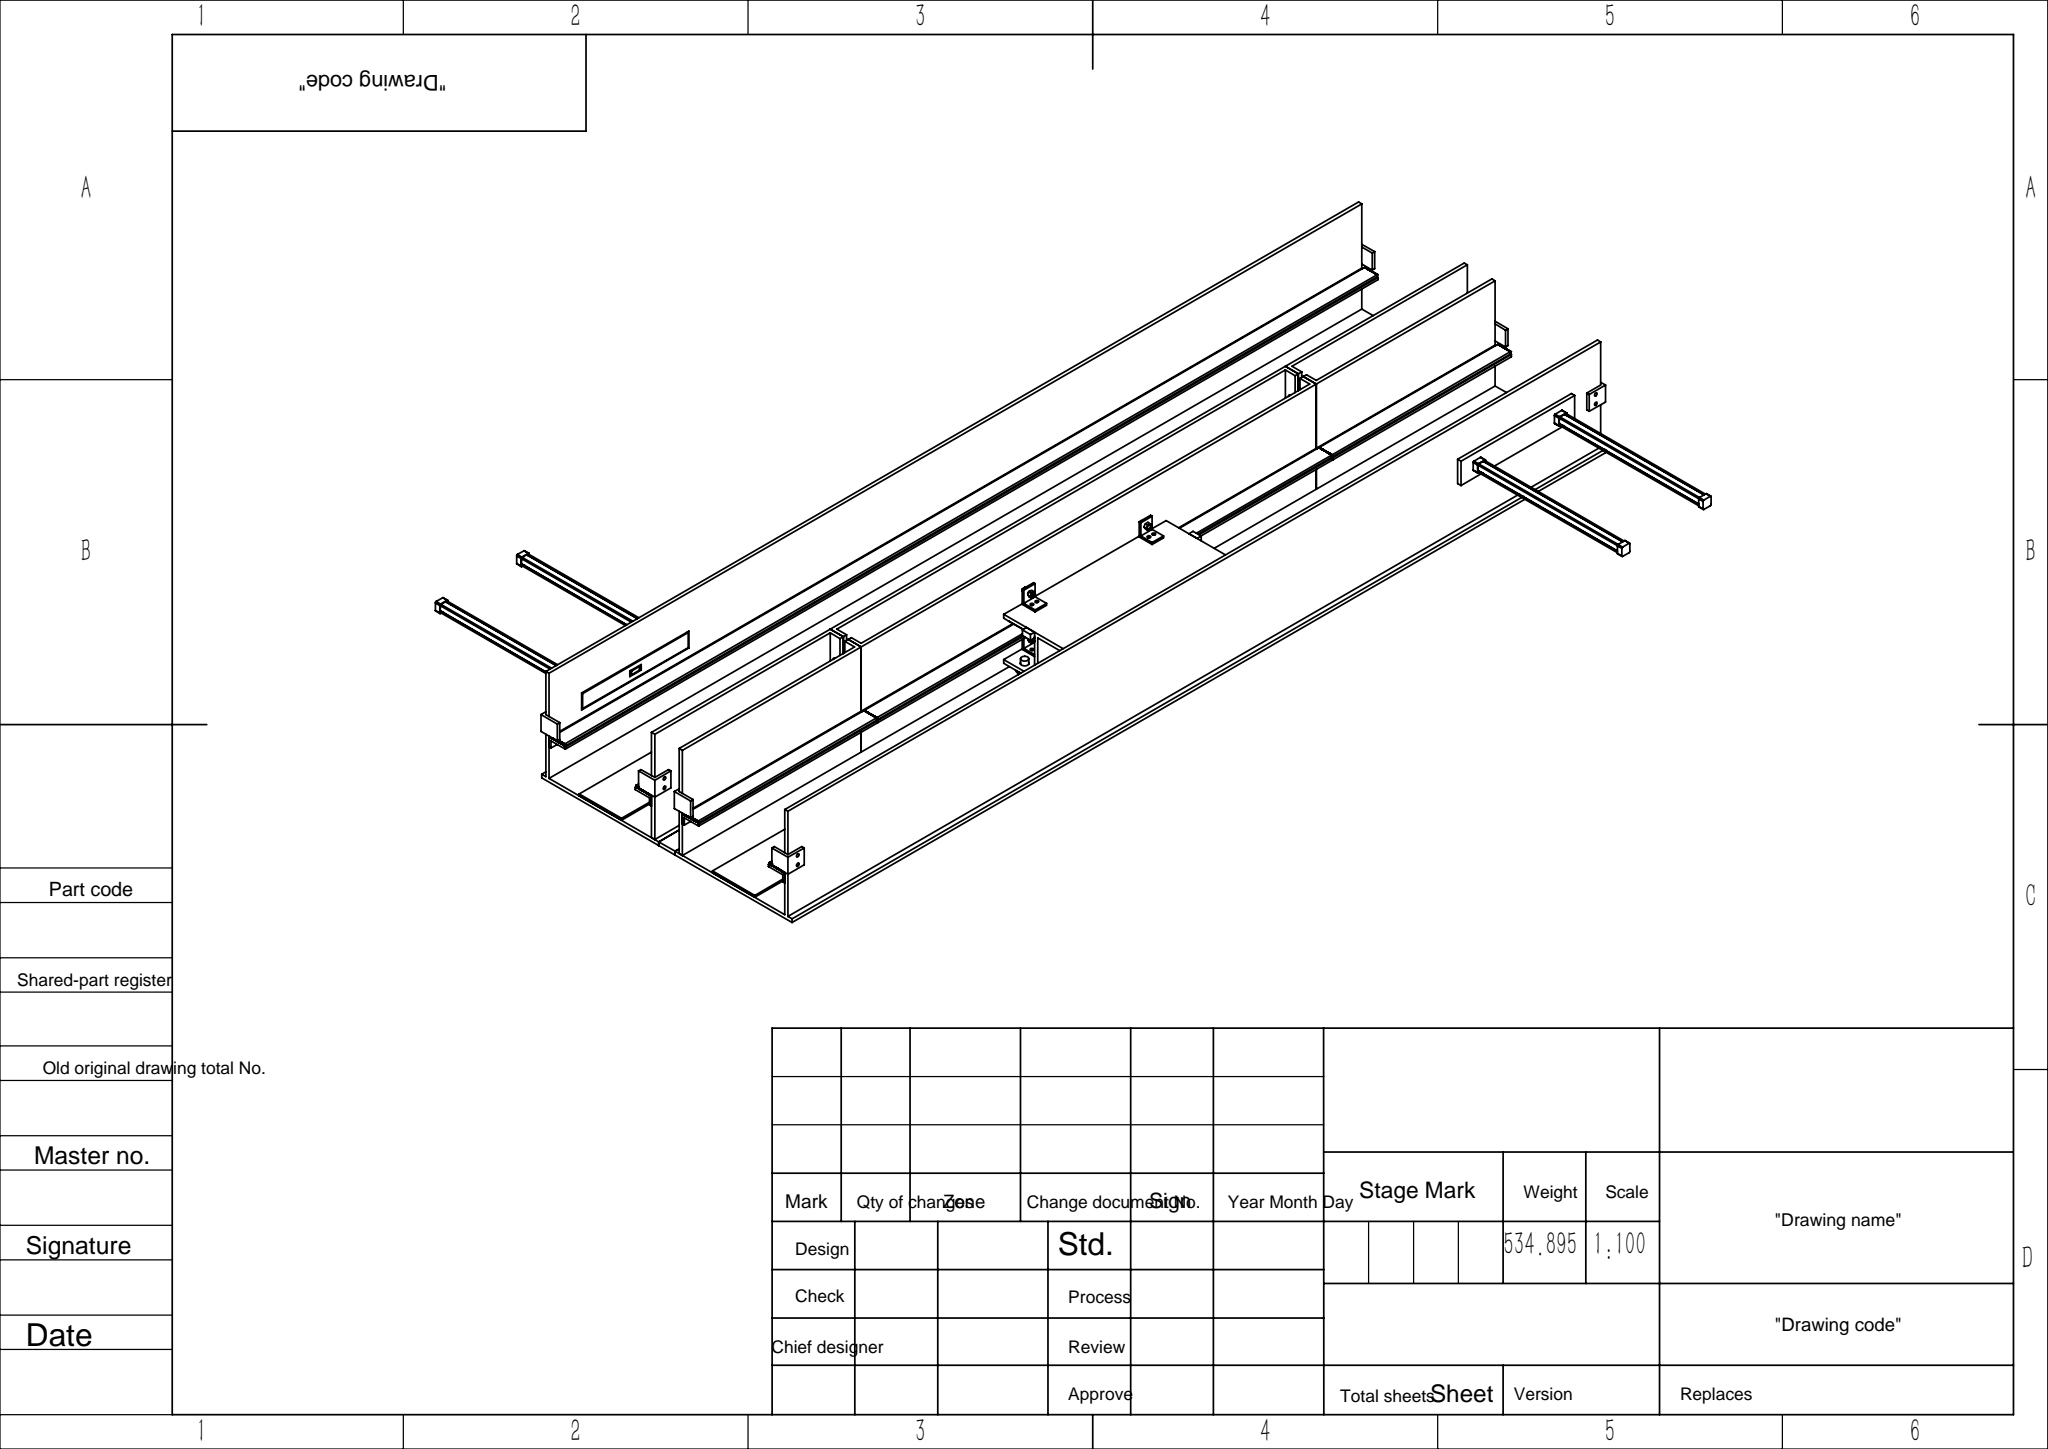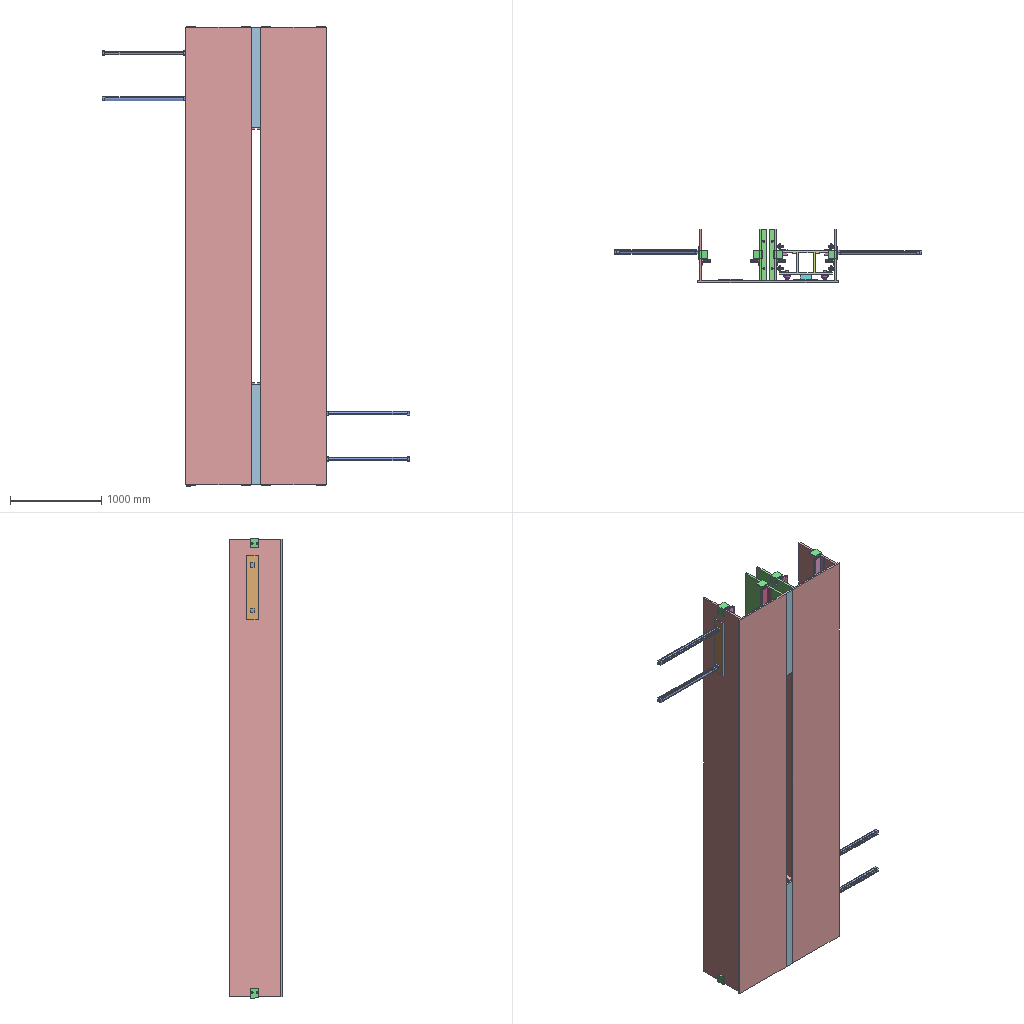Assembly | SolidWorks | 22 different items | 79 placed | box 3360 x 580 x 5030 mm
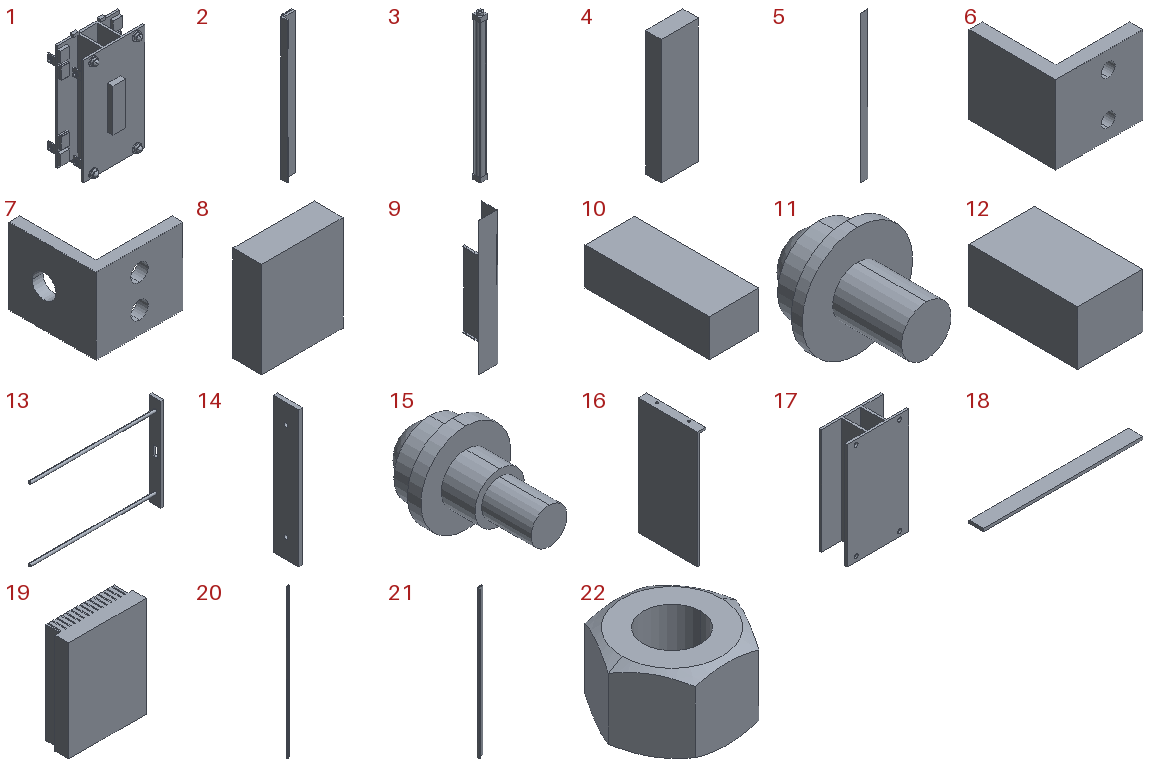Parts list (item | name | quantity | parent item | size | volume | features):
1 | (subassembly) | x1 | - | 626.912 x 393.248 x 1050 mm | 38288962 mm3 | features ReferencePattern 12, LocalLPattern 1
2 | - | x4 | - | 100 x 62 x 1100 mm | 2851141 mm3 | features ICE 3, Extrusion 1, LPattern 1, MirrorPattern 1
3 | - | x4 | - | 50 x 50 x 930 mm | 585630 mm3 | features ICE 5, Extrusion 1, Fillet 1
4 | - | x1 | in 1 | 120 x 50 x 400 mm | 2400000 mm3 | features Extrusion 1
5 | - | x2 | - | 260 x 10 x 5000 mm | 13000000 mm3 | features Extrusion 1
6 | - | x8 | - | 100 x 100 x 90 mm | 243718 mm3 | features Extrusion 1, ICE 1
7 | - | x8 | in 1 | 80 x 80 x 70 mm | 97177 mm3 | features ICE 2, Extrusion 1
8 | - | x4 | in 1 | 85 x 30 x 100 mm | 255000 mm3 | features Extrusion 1
9 | - | x2 | - | 755 x 580 x 5000 mm | 159485589 mm3 | features ICE 4, Extrusion 1
10 | - | x2 | - | 20 x 50 x 15 mm | 15000 mm3 | features Extrusion 1
11 | - | x4 | in 1 | 80 x 98 x 80 mm | 170693 mm3 | features ICE 1, Revolution 1
12 | - | x4 | in 1 | 30 x 50 x 25 mm | 37500 mm3 | features Extrusion 1
13 | - | x2 | - | 900 x 80 x 650 mm | 1550920 mm3 | features ICE 2, Extrusion 1
14 | - | x2 | - | 20 x 130 x 700 mm | 1807434 mm3 | features Extrusion 1
15 | - | x8 | in 1 | 40 x 64 x 40 mm | 29255 mm3 | features ICE 2, Revolution 1
16 | - | x4 | - | 80 x 560 x 1100 mm | 12976795 mm3 | features ICE 3, Extrusion 1
17 | - | x1 | in 1 | 580 x 260 x 1000 mm | 31909271 mm3 | features Extrusion 1, ICE 1
18 | - | x2 | - | 1100 x 100 x 20 mm | 2200000 mm3 | features Extrusion 1
19 | - | x4 | in 1 | 85 x 30 x 110 mm | 263886 mm3 | features ICE 2, Extrusion 1, LPattern 1, MirrorPattern 1
20 | - | x2 | - | 100 x 62 x 5000 mm | 12959941 mm3 | features ICE 3, Extrusion 1, LPattern 1, MirrorPattern 1
21 | - | x2 | - | 100 x 62 x 2800 mm | 7257541 mm3 | features ICE 3, Extrusion 1, LPattern 1, MirrorPattern 1
22 | - | x8 | in 1 | 9.238 x 8 x 5.6 mm | 229.89 mm3 | features RevCut 2, Extrusion 1, LPattern 1
Mates (type | each side: item.copy, entity, surface, feature):
In the top assembly
Concentric | 3.1 face cylinder Boss-Extrude4 | 14.1 face cylinder Boss-Extrude1
Concentric | 3.2 face cylinder Boss-Extrude4 | 14.1 face cylinder Boss-Extrude1
Coincident | 14.1 face plane Boss-Extrude1 | 3.2 face plane Boss-Extrude3
Coincident | 3.1 face plane Boss-Extrude3 | 3.2 face plane Boss-Extrude3
Parallel | 9.1 face plane Boss-Extrude1 | 13.1 face plane Cut-Extrude1
Coincident | 9.1 face plane Boss-Extrude1 | 9.2 face plane Boss-Extrude1 | 2 times
DistanceDim | 9.2 face plane Boss-Extrude1 | 9.1 face plane Boss-Extrude1
Coincident | 3.3 face plane Boss-Extrude1 | 3.4 face plane Boss-Extrude1 | 2 times
Coincident | 14.2 face plane Boss-Extrude1 | 3.4 face plane Boss-Extrude3
Concentric | 3.4 face cylinder Boss-Extrude2 | 13.2 face cylinder Boss-Extrude2
Parallel | 9.2 face plane Boss-Extrude1 | 13.2 face plane Cut-Extrude1
Coincident | 9.1 face plane Boss-Extrude1 | 20.1 face plane Boss-Extrude1
Coincident | 9.2 face plane Boss-Extrude1 | 20.2 face plane Boss-Extrude1 | 2 times
Coincident | 20.1 face plane Boss-Extrude1 | 20.2 face plane Boss-Extrude1 | 2 times
Coincident | 9.2 face plane Boss-Extrude1 | 21.1 face plane Boss-Extrude1
Coincident | 20.2 face plane Boss-Extrude1 | 21.1 face plane Boss-Extrude1
Coincident | 9.1 face plane Boss-Extrude1 | 21.2 face plane Boss-Extrude1
Coincident | 20.1 face plane Boss-Extrude1 | 21.2 face plane Boss-Extrude1
Coincident | 9.1 face plane Boss-Extrude1 | 14.1 face plane Boss-Extrude1
DistanceDim | 14.1 face plane Boss-Extrude1 | 9.1 face plane Cut-Extrude1 | 2 times
Concentric | 13.1 face cylinder Boss-Extrude2 | 14.1 face cylinder Boss-Extrude1
Coincident | 3.1 face plane Boss-Extrude1 | 3.2 face plane Boss-Extrude1
Coincident | 9.2 face plane Boss-Extrude1 | 14.2 face plane Boss-Extrude1
DistanceDim | 14.2 face plane Boss-Extrude1 | 9.2 face plane Cut-Extrude1 | 2 times
Concentric | 3.3 face cylinder Boss-Extrude2 | 14.2 face cylinder Boss-Extrude1
Concentric | 3.3 face cylinder Boss-Extrude2 | 13.2 face cylinder Boss-Extrude2
Coincident | 9.2 face plane Boss-Extrude1 | 5.1 face plane Boss-Extrude1
Coincident | 9.1 face plane Boss-Extrude1 | 5.2 face plane Boss-Extrude1 | 2 times
DistanceDim | 5.2 face plane Boss-Extrude1 | 9.1 face plane Boss-Extrude1
Coincident | 9.2 face plane Boss-Extrude1 | 5.1 edge
DistanceDim | 5.1 face plane Boss-Extrude1 | 9.2 face plane Boss-Extrude1
Coincident | 16.1 face plane Boss-Extrude1 | 2.1 face plane Boss-Extrude1
Coincident | 21.1 face plane Boss-Extrude1 | 2.1 face plane Boss-Extrude1 | 2 times
Coincident | 9.2 face plane Boss-Extrude1 | 16.1 face plane Cut-Extrude1
Coincident | 9.2 face plane Cut-Extrude2 | 16.1 face plane Boss-Extrude1
Coincident | 9.2 face plane Boss-Extrude1 | 16.1 face plane Boss-Extrude1
Coincident | 16.2 face plane Boss-Extrude1 | 2.2 face plane Boss-Extrude1
Coincident | 21.1 face plane Boss-Extrude1 | 2.2 face plane Boss-Extrude1
Coincident | 9.2 face plane Boss-Extrude1 | 16.2 face plane Cut-Extrude1
Coincident | 9.2 face plane Cut-Extrude2 | 16.2 face plane Boss-Extrude1
Coincident | 9.1 face plane Boss-Extrude1 | 16.2 face plane Boss-Extrude1
Coincident | 9.2 face plane Cut-Extrude2 | 16.3 face plane Boss-Extrude1
Coincident | 9.2 face plane Boss-Extrude1 | 16.3 face plane Boss-Extrude1
Coincident | 9.2 face plane Boss-Extrude1 | 16.3 face plane Cut-Extrude1
Coincident | 16.3 face plane Boss-Extrude1 | 2.3 face plane Boss-Extrude1
Coincident | 21.1 face plane Boss-Extrude1 | 2.3 face plane Boss-Extrude1 | 2 times
Coincident | 9.1 face plane Cut-Extrude2 | 16.4 face plane Boss-Extrude1
Coincident | 9.1 face plane Boss-Extrude1 | 16.4 face plane Boss-Extrude1
Coincident | 9.1 face plane Boss-Extrude1 | 16.4 face plane Cut-Extrude1
Coincident | 16.4 face plane Boss-Extrude1 | 2.4 face plane Boss-Extrude1
Coincident | 21.2 face plane Boss-Extrude1 | 2.4 face plane Boss-Extrude1 | 2 times
Coincident | 9.1 face plane Boss-Extrude1 | 18.1 face plane Boss-Extrude1 | 3 times
Coincident | 9.2 face plane Boss-Extrude1 | 18.2 face plane Boss-Extrude1 | 3 times
Coincident | 13.1 face plane Boss-Extrude1 | 17.1 face plane Boss-Extrude1
DistanceDim | 17.1 face plane Boss-Extrude1 | 9.1 face plane Boss-Extrude1
Coincident | 13.1 face plane Boss-Extrude1 | 10.1 face plane Boss-Extrude1
DistanceDim | 10.1 face plane Boss-Extrude1 | 13.1 face plane Boss-Extrude1 | 2 times
DistanceDim | 10.2 face plane Boss-Extrude1 | 13.2 face plane Boss-Extrude1 | 2 times
Coincident | 13.2 face plane Boss-Extrude1 | 10.2 face plane Boss-Extrude1
DistanceDim | 20.2 face plane Boss-Extrude1 | 9.2 face plane Boss-Extrude1
Coincident | 20.2 face plane Boss-Extrude1 | 2.2 face plane Boss-Extrude1
Coincident | 21.2 face plane Boss-Extrude1 | 2.2 face plane Boss-Extrude1
Coincident | 20.2 face plane Boss-Extrude1 | 2.3 face plane Boss-Extrude1
Coincident | 9.2 face plane Boss-Extrude1 | 6.1 face plane Boss-Extrude1 | 2 times
DistanceDim | 6.1 face plane Boss-Extrude1 | 9.2 face plane Boss-Extrude1
Coincident | 9.2 face plane Boss-Extrude1 | 6.2 face plane Boss-Extrude1 | 2 times
Coincident | 6.1 face plane Boss-Extrude1 | 6.2 face plane Boss-Extrude1
Coincident | 16.1 face plane Boss-Extrude1 | 6.3 face plane Boss-Extrude1
Coincident | 6.2 face plane Boss-Extrude1 | 6.3 face plane Boss-Extrude1 | 2 times
Coincident | 6.3 face plane Boss-Extrude1 | 6.4 face plane Boss-Extrude1 | 2 times
Coincident | 16.4 face plane Boss-Extrude1 | 6.4 face plane Boss-Extrude1
Coincident | 6.4 face plane Boss-Extrude1 | 6.5 face plane Boss-Extrude1 | 2 times
Coincident | 9.1 face plane Boss-Extrude1 | 6.5 face plane Boss-Extrude1
Coincident | 6.1 face plane Boss-Extrude1 | 6.6 face plane Boss-Extrude1 | 2 times
Coincident | 6.6 face plane Boss-Extrude1 | 6.7 face plane Boss-Extrude1 | 2 times
Coincident | 6.7 face plane Boss-Extrude1 | 6.8 face plane Boss-Extrude1 | 2 times
Coincident | 6.5 face plane Boss-Extrude1 | 6.8 face plane Boss-Extrude1
Coincident | 6.4 face plane Boss-Extrude1 | 6.7 face plane Boss-Extrude1
Coincident | 6.3 face plane Boss-Extrude1 | 6.6 face plane Boss-Extrude1
In subassembly 1
Concentric | 17.2 face cylinder Cut-Extrude1 | 11.1 face cylinder Boss-Extrude1
Concentric | 17.2 face cylinder Cut-Extrude1 | 11.2 face cylinder Boss-Extrude1
Concentric | 17.2 face cylinder Cut-Extrude1 | 11.3 face cylinder Boss-Extrude1
Concentric | 17.2 face cylinder Cut-Extrude1 | 11.4 face cylinder Boss-Extrude1
Coincident | 11.3 face plane Revolve1 | 11.4 face plane Revolve1
Coincident | 11.2 face plane Revolve1 | 11.4 face plane Revolve1
Coincident | 11.1 face plane Revolve1 | 11.2 face plane Revolve1
Coincident | 17.2 face plane Boss-Extrude1 | 7.1 face plane Boss-Extrude1
Concentric | 7.1 face cylinder Cut-Extrude2 | 15.1 face cylinder Boss-Extrude2
Coincident | 7.1 face plane Boss-Extrude1 | 15.1 face plane Revolve1
DistanceDim | 7.1 face plane Boss-Extrude1 | 17.2 face plane Boss-Extrude1
Concentric | 7.2 face cylinder Cut-Extrude2 | 15.2 face cylinder Boss-Extrude1
Coincident | 7.2 face plane Boss-Extrude1 | 15.2 face plane Revolve1
Coincident | 7.1 face plane Boss-Extrude1 | 7.2 face plane Boss-Extrude1 | 2 times
Concentric | 15.1 face cylinder Boss-Extrude2 | 22.1 face cylinder BaseNut
Coincident | 7.1 face plane Boss-Extrude1 | 22.1 face plane BaseNut
Concentric | 15.2 face cylinder Boss-Extrude2 | 22.2 face cylinder BaseNut
Coincident | 7.2 face plane Boss-Extrude1 | 22.2 face plane BaseNut
Coincident | 17.2 face plane Boss-Extrude1 | 19.1 face plane Boss-Extrude1 | 2 times
Coincident | 17.2 face plane Boss-Extrude1 | 19.2 face plane Boss-Extrude1 | 2 times
Coincident | 17.2 face plane Boss-Extrude1 | 19.3 face plane Boss-Extrude1 | 2 times
Coincident | 17.2 face plane Boss-Extrude1 | 19.4 face plane Boss-Extrude1 | 2 times
Coincident | 8.1 face plane Boss-Extrude1 | 17.2 face plane Boss-Extrude1
Coincident | 17.2 face plane Boss-Extrude1 | 8.2 face plane Boss-Extrude1 | 2 times
Coincident | 17.2 face plane Boss-Extrude1 | 8.3 face plane Boss-Extrude1 | 2 times
Coincident | 4.1 face plane Boss-Extrude1 | 17.2 face plane Boss-Extrude1
DistanceDim | 4.1 face plane Boss-Extrude1 | 17.2 face plane Boss-Extrude1 | 2 times
Coincident | 17.2 face plane Boss-Extrude1 | 12.1 face plane Boss-Extrude1 | 3 times
Coincident | 17.2 face plane Boss-Extrude1 | 12.2 face plane Boss-Extrude1 | 3 times
Coincident | 17.2 face plane Boss-Extrude1 | 12.3 face plane Boss-Extrude1 | 3 times
Coincident | 17.2 face plane Boss-Extrude1 | 12.4 face plane Boss-Extrude1 | 3 times
Concentric | 15.3 face cylinder Revolve1 | 7.3 face cylinder Cut-Extrude2
Concentric | 15.3 face cylinder Boss-Extrude2 | 22.3 face cylinder BaseNut
Concentric | 15.4 face cylinder Boss-Extrude2 | 7.4 face cylinder Cut-Extrude2
Concentric | 15.4 face cylinder Boss-Extrude2 | 22.4 face cylinder BaseNut
Coincident | 19.2 face plane Boss-Extrude1 | 19.4 face plane Boss-Extrude1
Coincident | 17.2 face plane Boss-Extrude1 | 8.4 face plane Boss-Extrude1 | 2 times
Coincident | 17.2 face plane Boss-Extrude1 | 8.1 face plane Boss-Extrude1
DistanceDim | 8.1 face plane Boss-Extrude1 | 17.2 face plane Boss-Extrude1
Coincident | 19.1 face plane Boss-Extrude1 | 19.3 face plane Boss-Extrude1
Coincident | 8.1 face plane Boss-Extrude1 | 8.3 face plane Boss-Extrude1
DistanceDim | 19.3 face plane Boss-Extrude1 | 8.1 face plane Boss-Extrude1
DistanceDim | 8.2 face plane Boss-Extrude1 | 17.2 face plane Boss-Extrude1
DistanceDim | 8.2 face plane Boss-Extrude1 | 19.4 face plane Boss-Extrude1
Coincident | 8.2 edge | 8.4 face plane Boss-Extrude1